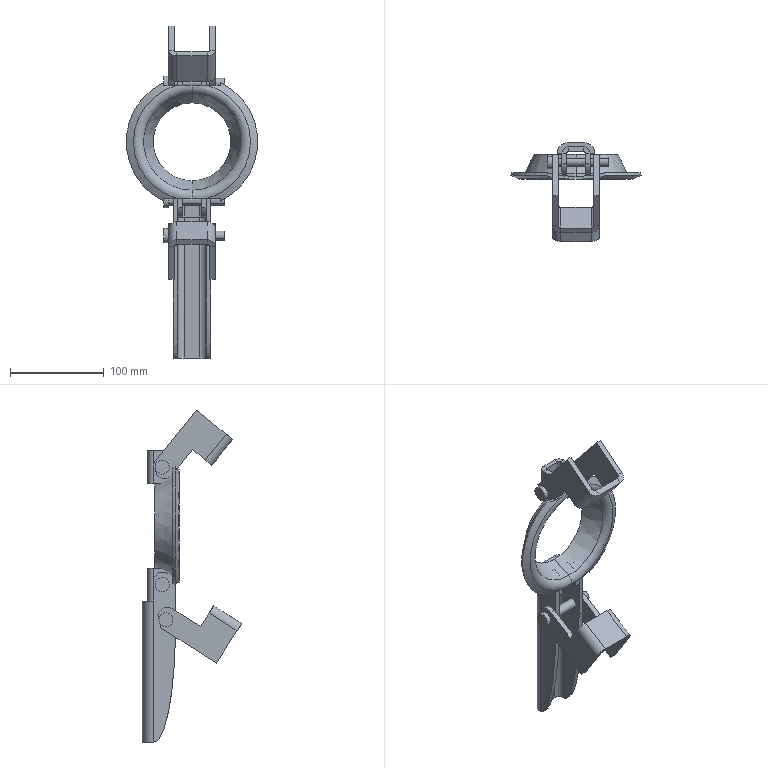Part | SolidWorks | features BaseBody 9 | 9 solids | 196 faces | box 140 x 105.523 x 353.223 mm | volume 225582 mm3 | plane 110 | cylinder 70 | cone 10 | torus 4 | spline 2 | commonest cylinder face diameters 10 x22 11 x8 36.097 x8 14 x6 15 x6 20 x6